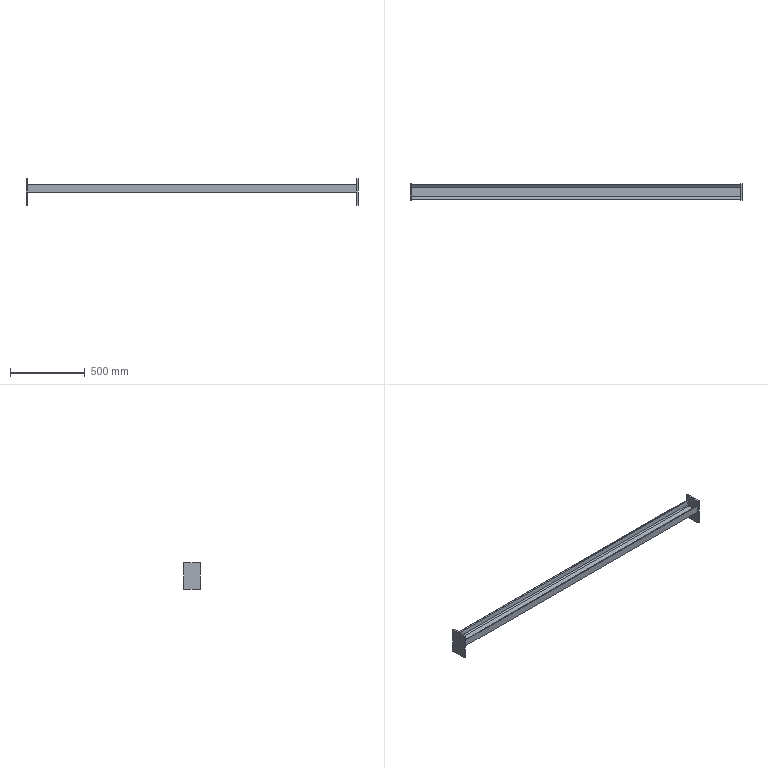Part | STEP file | Cross beam_Default<Machined> | 3 solids | 26 faces | box 2220 x 107.726 x 177.73 mm | volume 3150772 mm3 | plane 22 | cylinder 4 | commonest cylinder face diameters 8.5 x2 17 x2
STEP:
#1=CARTESIAN_POINT('',(-1100.,-100.,48.));
#2=VERTEX_POINT('',#1);
#3=CARTESIAN_POINT('',(-1100.,-100.,0.));
#4=VERTEX_POINT('',#3);
#5=CARTESIAN_POINT('',(-1100.,-100.,0.));
#6=DIRECTION('',(0.,0.,-1.));
#7=VECTOR('',#6,1000.);
#8=LINE('',#5,#7);
#9=EDGE_CURVE('',#2,#4,#8,.T.);
#10=ORIENTED_EDGE('',*,*,#9,.T.);
#11=CARTESIAN_POINT('',(1100.,-100.,0.));
#12=VERTEX_POINT('',#11);
#13=CARTESIAN_POINT('',(1100.,-100.,0.));
#14=DIRECTION('',(-1.,0.,0.));
#15=VECTOR('',#14,1000.);
#16=LINE('',#13,#15);
#17=EDGE_CURVE('',#12,#4,#16,.T.);
#18=ORIENTED_EDGE('',*,*,#17,.F.);
#19=CARTESIAN_POINT('',(1100.,-100.,48.));
#20=VERTEX_POINT('',#19);
#21=CARTESIAN_POINT('',(1100.,-100.,0.));
#22=DIRECTION('',(0.,0.,-1.));
#23=VECTOR('',#22,1000.);
#24=LINE('',#21,#23);
#25=EDGE_CURVE('',#20,#12,#24,.T.);
#26=ORIENTED_EDGE('',*,*,#25,.F.);
#27=CARTESIAN_POINT('',(1100.,-100.,48.));
#28=DIRECTION('',(-1.,0.,0.));
#29=VECTOR('',#28,1000.);
#30=LINE('',#27,#29);
#31=EDGE_CURVE('',#20,#2,#30,.T.);
#32=ORIENTED_EDGE('',*,*,#31,.T.);
#33=EDGE_LOOP('',(#10,#18,#26,#32));
#34=FACE_OUTER_BOUND('',#33,.T.);
#35=CARTESIAN_POINT('',(1100.,-100.,0.));
#36=DIRECTION('',(0.,1.,0.));
#37=DIRECTION('',(0.,0.,1.));
#38=AXIS2_PLACEMENT_3D('',#35,#36,#37);
#39=PLANE('',#38);
#40=ADVANCED_FACE('',(#34),#39,.F.);
#41=CARTESIAN_POINT('',(-1100.,0.,0.));
#42=VERTEX_POINT('',#41);
#43=CARTESIAN_POINT('',(-1100.,0.,0.));
#44=DIRECTION('',(0.,1.,0.));
#45=VECTOR('',#44,1000.);
#46=LINE('',#43,#45);
#47=EDGE_CURVE('',#4,#42,#46,.T.);
#48=ORIENTED_EDGE('',*,*,#47,.T.);
#49=CARTESIAN_POINT('',(1100.,0.,0.));
#50=VERTEX_POINT('',#49);
#51=CARTESIAN_POINT('',(1100.,0.,0.));
#52=DIRECTION('',(-1.,0.,0.));
#53=VECTOR('',#52,1000.);
#54=LINE('',#51,#53);
#55=EDGE_CURVE('',#50,#42,#54,.T.);
#56=ORIENTED_EDGE('',*,*,#55,.F.);
#57=CARTESIAN_POINT('',(1100.,0.,0.));
#58=DIRECTION('',(0.,1.,0.));
#59=VECTOR('',#58,1000.);
#60=LINE('',#57,#59);
#61=EDGE_CURVE('',#12,#50,#60,.T.);
#62=ORIENTED_EDGE('',*,*,#61,.F.);
#63=ORIENTED_EDGE('',*,*,#17,.T.);
#64=EDGE_LOOP('',(#48,#56,#62,#63));
#65=FACE_OUTER_BOUND('',#64,.T.);
#66=CARTESIAN_POINT('',(1100.,0.,0.));
#67=DIRECTION('',(0.,0.,1.));
#68=DIRECTION('',(1.,0.,0.));
#69=AXIS2_PLACEMENT_3D('',#66,#67,#68);
#70=PLANE('',#69);
#71=ADVANCED_FACE('',(#65),#70,.F.);
#72=CARTESIAN_POINT('',(-1100.,0.,48.));
#73=VERTEX_POINT('',#72);
#74=CARTESIAN_POINT('',(-1100.,0.,0.));
#75=DIRECTION('',(0.,0.,1.));
#76=VECTOR('',#75,1000.);
#77=LINE('',#74,#76);
#78=EDGE_CURVE('',#42,#73,#77,.T.);
#79=ORIENTED_EDGE('',*,*,#78,.T.);
#80=CARTESIAN_POINT('',(1100.,0.,48.));
#81=VERTEX_POINT('',#80);
#82=CARTESIAN_POINT('',(1100.,0.,48.));
#83=DIRECTION('',(-1.,0.,0.));
#84=VECTOR('',#83,1000.);
#85=LINE('',#82,#84);
#86=EDGE_CURVE('',#81,#73,#85,.T.);
#87=ORIENTED_EDGE('',*,*,#86,.F.);
#88=CARTESIAN_POINT('',(1100.,0.,0.));
#89=DIRECTION('',(0.,0.,1.));
#90=VECTOR('',#89,1000.);
#91=LINE('',#88,#90);
#92=EDGE_CURVE('',#50,#81,#91,.T.);
#93=ORIENTED_EDGE('',*,*,#92,.F.);
#94=ORIENTED_EDGE('',*,*,#55,.T.);
#95=EDGE_LOOP('',(#79,#87,#93,#94));
#96=FACE_OUTER_BOUND('',#95,.T.);
#97=CARTESIAN_POINT('',(1100.,0.,0.));
#98=DIRECTION('',(0.,-1.,0.));
#99=DIRECTION('',(0.,0.,-1.));
#100=AXIS2_PLACEMENT_3D('',#97,#98,#99);
#101=PLANE('',#100);
#102=ADVANCED_FACE('',(#96),#101,.F.);
#103=CARTESIAN_POINT('',(-1100.,-2.734,48.));
#104=VERTEX_POINT('',#103);
#105=CARTESIAN_POINT('',(-1100.,-2.734,48.));
#106=DIRECTION('',(0.,-1.,0.));
#107=VECTOR('',#106,1000.);
#108=LINE('',#105,#107);
#109=EDGE_CURVE('',#73,#104,#108,.T.);
#110=ORIENTED_EDGE('',*,*,#109,.T.);
#111=CARTESIAN_POINT('',(1100.,-2.734,48.));
#112=VERTEX_POINT('',#111);
#113=CARTESIAN_POINT('',(1100.,-2.734,48.));
#114=DIRECTION('',(-1.,0.,0.));
#115=VECTOR('',#114,1000.);
#116=LINE('',#113,#115);
#117=EDGE_CURVE('',#112,#104,#116,.T.);
#118=ORIENTED_EDGE('',*,*,#117,.F.);
#119=CARTESIAN_POINT('',(1100.,-2.734,48.));
#120=DIRECTION('',(0.,-1.,0.));
#121=VECTOR('',#120,1000.);
#122=LINE('',#119,#121);
#123=EDGE_CURVE('',#81,#112,#122,.T.);
#124=ORIENTED_EDGE('',*,*,#123,.F.);
#125=ORIENTED_EDGE('',*,*,#86,.T.);
#126=EDGE_LOOP('',(#110,#118,#124,#125));
#127=FACE_OUTER_BOUND('',#126,.T.);
#128=CARTESIAN_POINT('',(1100.,-2.734,48.));
#129=DIRECTION('',(0.,0.,-1.));
#130=DIRECTION('',(0.,1.,0.));
#131=AXIS2_PLACEMENT_3D('',#128,#129,#130);
#132=PLANE('',#131);
#133=ADVANCED_FACE('',(#127),#132,.F.);
#134=CARTESIAN_POINT('',(-1100.,-6.972,44.073));
#135=VERTEX_POINT('',#134);
#136=CARTESIAN_POINT('',(-1100.,-2.734,43.75));
#137=DIRECTION('',(1.,0.,0.));
#138=DIRECTION('',(0.,0.,-1.));
#139=AXIS2_PLACEMENT_3D('',#136,#137,#138);
#140=CIRCLE('',#139,4.25);
#141=EDGE_CURVE('',#104,#135,#140,.T.);
#142=ORIENTED_EDGE('',*,*,#141,.T.);
#143=CARTESIAN_POINT('',(1100.,-6.972,44.073));
#144=VERTEX_POINT('',#143);
#145=CARTESIAN_POINT('',(1100.,-6.972,44.073));
#146=DIRECTION('',(-1.,0.,0.));
#147=VECTOR('',#146,1000.);
#148=LINE('',#145,#147);
#149=EDGE_CURVE('',#144,#135,#148,.T.);
#150=ORIENTED_EDGE('',*,*,#149,.F.);
#151=CARTESIAN_POINT('',(1100.,-2.734,43.75));
#152=DIRECTION('',(1.,0.,0.));
#153=DIRECTION('',(0.,0.,-1.));
#154=AXIS2_PLACEMENT_3D('',#151,#152,#153);
#155=CIRCLE('',#154,4.25);
#156=EDGE_CURVE('',#112,#144,#155,.T.);
#157=ORIENTED_EDGE('',*,*,#156,.F.);
#158=ORIENTED_EDGE('',*,*,#117,.T.);
#159=EDGE_LOOP('',(#142,#150,#157,#158));
#160=FACE_OUTER_BOUND('',#159,.T.);
#161=CARTESIAN_POINT('',(1100.,-2.734,43.75));
#162=DIRECTION('',(-1.,0.,0.));
#163=DIRECTION('',(0.,0.,1.));
#164=AXIS2_PLACEMENT_3D('',#161,#162,#163);
#165=CYLINDRICAL_SURFACE('',#164,4.25);
#166=ADVANCED_FACE('',(#160),#165,.T.);
#167=CARTESIAN_POINT('',(-1100.,-9.325,13.155));
#168=VERTEX_POINT('',#167);
#169=CARTESIAN_POINT('',(-1100.,-9.325,13.155));
#170=DIRECTION('',(0.,-0.07589,-0.9971));
#171=VECTOR('',#170,1000.);
#172=LINE('',#169,#171);
#173=EDGE_CURVE('',#135,#168,#172,.T.);
#174=ORIENTED_EDGE('',*,*,#173,.T.);
#175=CARTESIAN_POINT('',(1100.,-9.325,13.155));
#176=VERTEX_POINT('',#175);
#177=CARTESIAN_POINT('',(1100.,-9.325,13.155));
#178=DIRECTION('',(-1.,0.,0.));
#179=VECTOR('',#178,1000.);
#180=LINE('',#177,#179);
#181=EDGE_CURVE('',#176,#168,#180,.T.);
#182=ORIENTED_EDGE('',*,*,#181,.F.);
#183=CARTESIAN_POINT('',(1100.,-9.325,13.155));
#184=DIRECTION('',(0.,-0.07589,-0.9971));
#185=VECTOR('',#184,1000.);
#186=LINE('',#183,#185);
#187=EDGE_CURVE('',#144,#176,#186,.T.);
#188=ORIENTED_EDGE('',*,*,#187,.F.);
#189=ORIENTED_EDGE('',*,*,#149,.T.);
#190=EDGE_LOOP('',(#174,#182,#188,#189));
#191=FACE_OUTER_BOUND('',#190,.T.);
#192=CARTESIAN_POINT('',(1100.,-9.325,13.155));
#193=DIRECTION('',(0.,0.9971,-0.07589));
#194=DIRECTION('',(0.,0.07589,0.9971));
#195=AXIS2_PLACEMENT_3D('',#192,#193,#194);
#196=PLANE('',#195);
#197=ADVANCED_FACE('',(#191),#196,.F.);
#198=CARTESIAN_POINT('',(-1100.,-17.801,5.3));
#199=VERTEX_POINT('',#198);
#200=CARTESIAN_POINT('',(-1100.,-17.801,13.8));
#201=DIRECTION('',(-1.,0.,0.));
#202=DIRECTION('',(0.,0.,1.));
#203=AXIS2_PLACEMENT_3D('',#200,#201,#202);
#204=CIRCLE('',#203,8.5);
#205=EDGE_CURVE('',#168,#199,#204,.T.);
#206=ORIENTED_EDGE('',*,*,#205,.T.);
#207=CARTESIAN_POINT('',(1100.,-17.801,5.3));
#208=VERTEX_POINT('',#207);
#209=CARTESIAN_POINT('',(1100.,-17.801,5.3));
#210=DIRECTION('',(-1.,0.,0.));
#211=VECTOR('',#210,1000.);
#212=LINE('',#209,#211);
#213=EDGE_CURVE('',#208,#199,#212,.T.);
#214=ORIENTED_EDGE('',*,*,#213,.F.);
#215=CARTESIAN_POINT('',(1100.,-17.801,13.8));
#216=DIRECTION('',(-1.,0.,0.));
#217=DIRECTION('',(0.,0.,1.));
#218=AXIS2_PLACEMENT_3D('',#215,#216,#217);
#219=CIRCLE('',#218,8.5);
#220=EDGE_CURVE('',#176,#208,#219,.T.);
#221=ORIENTED_EDGE('',*,*,#220,.F.);
#222=ORIENTED_EDGE('',*,*,#181,.T.);
#223=EDGE_LOOP('',(#206,#214,#221,#222));
#224=FACE_OUTER_BOUND('',#223,.T.);
#225=CARTESIAN_POINT('',(1100.,-17.801,13.8));
#226=DIRECTION('',(-1.,0.,0.));
#227=DIRECTION('',(0.,0.,1.));
#228=AXIS2_PLACEMENT_3D('',#225,#226,#227);
#229=CYLINDRICAL_SURFACE('',#228,8.5);
#230=ADVANCED_FACE('',(#224),#229,.F.);
#231=CARTESIAN_POINT('',(-1100.,-82.199,5.3));
#232=VERTEX_POINT('',#231);
#233=CARTESIAN_POINT('',(-1100.,-82.199,5.3));
#234=DIRECTION('',(0.,-1.,0.));
#235=VECTOR('',#234,1000.);
#236=LINE('',#233,#235);
#237=EDGE_CURVE('',#199,#232,#236,.T.);
#238=ORIENTED_EDGE('',*,*,#237,.T.);
#239=CARTESIAN_POINT('',(1100.,-82.199,5.3));
#240=VERTEX_POINT('',#239);
#241=CARTESIAN_POINT('',(1100.,-82.199,5.3));
#242=DIRECTION('',(-1.,0.,0.));
#243=VECTOR('',#242,1000.);
#244=LINE('',#241,#243);
#245=EDGE_CURVE('',#240,#232,#244,.T.);
#246=ORIENTED_EDGE('',*,*,#245,.F.);
#247=CARTESIAN_POINT('',(1100.,-82.199,5.3));
#248=DIRECTION('',(0.,-1.,0.));
#249=VECTOR('',#248,1000.);
#250=LINE('',#247,#249);
#251=EDGE_CURVE('',#208,#240,#250,.T.);
#252=ORIENTED_EDGE('',*,*,#251,.F.);
#253=ORIENTED_EDGE('',*,*,#213,.T.);
#254=EDGE_LOOP('',(#238,#246,#252,#253));
#255=FACE_OUTER_BOUND('',#254,.T.);
#256=CARTESIAN_POINT('',(1100.,-82.199,5.3));
#257=DIRECTION('',(0.,0.,-1.));
#258=DIRECTION('',(-1.,0.,0.));
#259=AXIS2_PLACEMENT_3D('',#256,#257,#258);
#260=PLANE('',#259);
#261=ADVANCED_FACE('',(#255),#260,.F.);
#262=CARTESIAN_POINT('',(-1100.,-90.675,13.155));
#263=VERTEX_POINT('',#262);
#264=CARTESIAN_POINT('',(-1100.,-82.199,13.8));
#265=DIRECTION('',(-1.,0.,0.));
#266=DIRECTION('',(0.,0.,1.));
#267=AXIS2_PLACEMENT_3D('',#264,#265,#266);
#268=CIRCLE('',#267,8.5);
#269=EDGE_CURVE('',#232,#263,#268,.T.);
#270=ORIENTED_EDGE('',*,*,#269,.T.);
#271=CARTESIAN_POINT('',(1100.,-90.675,13.155));
#272=VERTEX_POINT('',#271);
#273=CARTESIAN_POINT('',(1100.,-90.675,13.155));
#274=DIRECTION('',(-1.,0.,0.));
#275=VECTOR('',#274,1000.);
#276=LINE('',#273,#275);
#277=EDGE_CURVE('',#272,#263,#276,.T.);
#278=ORIENTED_EDGE('',*,*,#277,.F.);
#279=CARTESIAN_POINT('',(1100.,-82.199,13.8));
#280=DIRECTION('',(-1.,0.,0.));
#281=DIRECTION('',(0.,0.,1.));
#282=AXIS2_PLACEMENT_3D('',#279,#280,#281);
#283=CIRCLE('',#282,8.5);
#284=EDGE_CURVE('',#240,#272,#283,.T.);
#285=ORIENTED_EDGE('',*,*,#284,.F.);
#286=ORIENTED_EDGE('',*,*,#245,.T.);
#287=EDGE_LOOP('',(#270,#278,#285,#286));
#288=FACE_OUTER_BOUND('',#287,.T.);
#289=CARTESIAN_POINT('',(1100.,-82.199,13.8));
#290=DIRECTION('',(-1.,0.,0.));
#291=DIRECTION('',(0.,0.,1.));
#292=AXIS2_PLACEMENT_3D('',#289,#290,#291);
#293=CYLINDRICAL_SURFACE('',#292,8.5);
#294=ADVANCED_FACE('',(#288),#293,.F.);
#295=CARTESIAN_POINT('',(-1100.,-93.028,44.073));
#296=VERTEX_POINT('',#295);
#297=CARTESIAN_POINT('',(-1100.,-90.675,13.155));
#298=DIRECTION('',(0.,-0.07589,0.9971));
#299=VECTOR('',#298,1000.);
#300=LINE('',#297,#299);
#301=EDGE_CURVE('',#263,#296,#300,.T.);
#302=ORIENTED_EDGE('',*,*,#301,.T.);
#303=CARTESIAN_POINT('',(1100.,-93.028,44.073));
#304=VERTEX_POINT('',#303);
#305=CARTESIAN_POINT('',(1100.,-93.028,44.073));
#306=DIRECTION('',(-1.,0.,0.));
#307=VECTOR('',#306,1000.);
#308=LINE('',#305,#307);
#309=EDGE_CURVE('',#304,#296,#308,.T.);
#310=ORIENTED_EDGE('',*,*,#309,.F.);
#311=CARTESIAN_POINT('',(1100.,-90.675,13.155));
#312=DIRECTION('',(0.,-0.07589,0.9971));
#313=VECTOR('',#312,1000.);
#314=LINE('',#311,#313);
#315=EDGE_CURVE('',#272,#304,#314,.T.);
#316=ORIENTED_EDGE('',*,*,#315,.F.);
#317=ORIENTED_EDGE('',*,*,#277,.T.);
#318=EDGE_LOOP('',(#302,#310,#316,#317));
#319=FACE_OUTER_BOUND('',#318,.T.);
#320=CARTESIAN_POINT('',(1100.,-90.675,13.155));
#321=DIRECTION('',(0.,-0.9971,-0.07589));
#322=DIRECTION('',(0.,0.07589,-0.9971));
#323=AXIS2_PLACEMENT_3D('',#320,#321,#322);
#324=PLANE('',#323);
#325=ADVANCED_FACE('',(#319),#324,.F.);
#326=CARTESIAN_POINT('',(-1100.,-97.266,48.));
#327=VERTEX_POINT('',#326);
#328=CARTESIAN_POINT('',(-1100.,-97.266,43.75));
#329=DIRECTION('',(1.,0.,0.));
#330=DIRECTION('',(0.,0.,-1.));
#331=AXIS2_PLACEMENT_3D('',#328,#329,#330);
#332=CIRCLE('',#331,4.25);
#333=EDGE_CURVE('',#296,#327,#332,.T.);
#334=ORIENTED_EDGE('',*,*,#333,.T.);
#335=CARTESIAN_POINT('',(1100.,-97.266,48.));
#336=VERTEX_POINT('',#335);
#337=CARTESIAN_POINT('',(1100.,-97.266,48.));
#338=DIRECTION('',(-1.,0.,0.));
#339=VECTOR('',#338,1000.);
#340=LINE('',#337,#339);
#341=EDGE_CURVE('',#336,#327,#340,.T.);
#342=ORIENTED_EDGE('',*,*,#341,.F.);
#343=CARTESIAN_POINT('',(1100.,-97.266,43.75));
#344=DIRECTION('',(1.,0.,0.));
#345=DIRECTION('',(0.,0.,-1.));
#346=AXIS2_PLACEMENT_3D('',#343,#344,#345);
#347=CIRCLE('',#346,4.25);
#348=EDGE_CURVE('',#304,#336,#347,.T.);
#349=ORIENTED_EDGE('',*,*,#348,.F.);
#350=ORIENTED_EDGE('',*,*,#309,.T.);
#351=EDGE_LOOP('',(#334,#342,#349,#350));
#352=FACE_OUTER_BOUND('',#351,.T.);
#353=CARTESIAN_POINT('',(1100.,-97.266,43.75));
#354=DIRECTION('',(-1.,0.,0.));
#355=DIRECTION('',(0.,0.,1.));
#356=AXIS2_PLACEMENT_3D('',#353,#354,#355);
#357=CYLINDRICAL_SURFACE('',#356,4.25);
#358=ADVANCED_FACE('',(#352),#357,.T.);
#359=CARTESIAN_POINT('',(-1100.,-97.266,48.));
#360=DIRECTION('',(0.,-1.,0.));
#361=VECTOR('',#360,1000.);
#362=LINE('',#359,#361);
#363=EDGE_CURVE('',#327,#2,#362,.T.);
#364=ORIENTED_EDGE('',*,*,#363,.T.);
#365=ORIENTED_EDGE('',*,*,#31,.F.);
#366=CARTESIAN_POINT('',(1100.,-97.266,48.));
#367=DIRECTION('',(0.,-1.,0.));
#368=VECTOR('',#367,1000.);
#369=LINE('',#366,#368);
#370=EDGE_CURVE('',#336,#20,#369,.T.);
#371=ORIENTED_EDGE('',*,*,#370,.F.);
#372=ORIENTED_EDGE('',*,*,#341,.T.);
#373=EDGE_LOOP('',(#364,#365,#371,#372));
#374=FACE_OUTER_BOUND('',#373,.T.);
#375=CARTESIAN_POINT('',(1100.,-97.266,48.));
#376=DIRECTION('',(0.,0.,-1.));
#377=DIRECTION('',(0.,1.,0.));
#378=AXIS2_PLACEMENT_3D('',#375,#376,#377);
#379=PLANE('',#378);
#380=ADVANCED_FACE('',(#374),#379,.F.);
#381=ORIENTED_EDGE('',*,*,#25,.T.);
#382=ORIENTED_EDGE('',*,*,#61,.T.);
#383=ORIENTED_EDGE('',*,*,#92,.T.);
#384=ORIENTED_EDGE('',*,*,#123,.T.);
#385=ORIENTED_EDGE('',*,*,#156,.T.);
#386=ORIENTED_EDGE('',*,*,#187,.T.);
#387=ORIENTED_EDGE('',*,*,#220,.T.);
#388=ORIENTED_EDGE('',*,*,#251,.T.);
#389=ORIENTED_EDGE('',*,*,#284,.T.);
#390=ORIENTED_EDGE('',*,*,#315,.T.);
#391=ORIENTED_EDGE('',*,*,#348,.T.);
#392=ORIENTED_EDGE('',*,*,#370,.T.);
#393=EDGE_LOOP('',(#381,#382,#383,#384,#385,#386,#387,#388,#389,#390,#391,#392));
#394=FACE_OUTER_BOUND('',#393,.T.);
#395=CARTESIAN_POINT('',(1100.,-97.266,43.75));
#396=DIRECTION('',(1.,0.,0.));
#397=DIRECTION('',(0.,0.,-1.));
#398=AXIS2_PLACEMENT_3D('',#395,#396,#397);
#399=PLANE('',#398);
#400=ADVANCED_FACE('',(#394),#399,.T.);
#401=ORIENTED_EDGE('',*,*,#9,.F.);
#402=ORIENTED_EDGE('',*,*,#363,.F.);
#403=ORIENTED_EDGE('',*,*,#333,.F.);
#404=ORIENTED_EDGE('',*,*,#301,.F.);
#405=ORIENTED_EDGE('',*,*,#269,.F.);
#406=ORIENTED_EDGE('',*,*,#237,.F.);
#407=ORIENTED_EDGE('',*,*,#205,.F.);
#408=ORIENTED_EDGE('',*,*,#173,.F.);
#409=ORIENTED_EDGE('',*,*,#141,.F.);
#410=ORIENTED_EDGE('',*,*,#109,.F.);
#411=ORIENTED_EDGE('',*,*,#78,.F.);
#412=ORIENTED_EDGE('',*,*,#47,.F.);
#413=EDGE_LOOP('',(#401,#402,#403,#404,#405,#406,#407,#408,#409,#410,#411,#412));
#414=FACE_OUTER_BOUND('',#413,.T.);
#415=CARTESIAN_POINT('',(-1100.,-97.266,43.75));
#416=DIRECTION('',(1.,0.,0.));
#417=DIRECTION('',(0.,0.,-1.));
#418=AXIS2_PLACEMENT_3D('',#415,#416,#417);
#419=PLANE('',#418);
#420=ADVANCED_FACE('',(#414),#419,.F.);
#421=CLOSED_SHELL('',(#40,#71,#102,#133,#166,#197,#230,#261,#294,#325,#358,#380,#400,#420));
#422=MANIFOLD_SOLID_BREP('',#421);
#423=CARTESIAN_POINT('',(-1100.,-103.863,88.865));
#424=VERTEX_POINT('',#423);
#425=CARTESIAN_POINT('',(-1100.,3.863,88.865));
#426=VERTEX_POINT('',#425);
#427=CARTESIAN_POINT('',(-1100.,-103.863,88.865));
#428=DIRECTION('',(0.,1.,0.));
#429=VECTOR('',#428,1000.);
#430=LINE('',#427,#429);
#431=EDGE_CURVE('',#424,#426,#430,.T.);
#432=ORIENTED_EDGE('',*,*,#431,.T.);
#433=CARTESIAN_POINT('',(-1110.,3.863,88.865));
#434=VERTEX_POINT('',#433);
#435=CARTESIAN_POINT('',(-1110.,3.863,88.865));
#436=DIRECTION('',(1.,0.,0.));
#437=VECTOR('',#436,1000.);
#438=LINE('',#435,#437);
#439=EDGE_CURVE('',#434,#426,#438,.T.);
#440=ORIENTED_EDGE('',*,*,#439,.F.);
#441=CARTESIAN_POINT('',(-1110.,-103.863,88.865));
#442=VERTEX_POINT('',#441);
#443=CARTESIAN_POINT('',(-1110.,-103.863,88.865));
#444=DIRECTION('',(0.,1.,0.));
#445=VECTOR('',#444,1000.);
#446=LINE('',#443,#445);
#447=EDGE_CURVE('',#442,#434,#446,.T.);
#448=ORIENTED_EDGE('',*,*,#447,.F.);
#449=CARTESIAN_POINT('',(-1110.,-103.863,88.865));
#450=DIRECTION('',(1.,0.,0.));
#451=VECTOR('',#450,1000.);
#452=LINE('',#449,#451);
#453=EDGE_CURVE('',#442,#424,#452,.T.);
#454=ORIENTED_EDGE('',*,*,#453,.T.);
#455=EDGE_LOOP('',(#432,#440,#448,#454));
#456=FACE_OUTER_BOUND('',#455,.T.);
#457=CARTESIAN_POINT('',(-1110.,-103.863,88.865));
#458=DIRECTION('',(0.,0.,-1.));
#459=DIRECTION('',(-1.,0.,0.));
#460=AXIS2_PLACEMENT_3D('',#457,#458,#459);
#461=PLANE('',#460);
#462=ADVANCED_FACE('',(#456),#461,.F.);
#463=CARTESIAN_POINT('',(-1100.,3.863,-88.865));
#464=VERTEX_POINT('',#463);
#465=CARTESIAN_POINT('',(-1100.,3.863,-88.865));
#466=DIRECTION('',(0.,0.,-1.));
#467=VECTOR('',#466,1000.);
#468=LINE('',#465,#467);
#469=EDGE_CURVE('',#426,#464,#468,.T.);
#470=ORIENTED_EDGE('',*,*,#469,.T.);
#471=CARTESIAN_POINT('',(-1110.,3.863,-88.865));
#472=VERTEX_POINT('',#471);
#473=CARTESIAN_POINT('',(-1110.,3.863,-88.865));
#474=DIRECTION('',(1.,0.,0.));
#475=VECTOR('',#474,1000.);
#476=LINE('',#473,#475);
#477=EDGE_CURVE('',#472,#464,#476,.T.);
#478=ORIENTED_EDGE('',*,*,#477,.F.);
#479=CARTESIAN_POINT('',(-1110.,3.863,-88.865));
#480=DIRECTION('',(0.,0.,-1.));
#481=VECTOR('',#480,1000.);
#482=LINE('',#479,#481);
#483=EDGE_CURVE('',#434,#472,#482,.T.);
#484=ORIENTED_EDGE('',*,*,#483,.F.);
#485=ORIENTED_EDGE('',*,*,#439,.T.);
#486=EDGE_LOOP('',(#470,#478,#484,#485));
#487=FACE_OUTER_BOUND('',#486,.T.);
#488=CARTESIAN_POINT('',(-1110.,3.863,-88.865));
#489=DIRECTION('',(0.,-1.,0.));
#490=DIRECTION('',(0.,0.,-1.));
#491=AXIS2_PLACEMENT_3D('',#488,#489,#490);
#492=PLANE('',#491);
#493=ADVANCED_FACE('',(#487),#492,.F.);
#494=CARTESIAN_POINT('',(-1100.,-103.863,-88.865));
#495=VERTEX_POINT('',#494);
#496=CARTESIAN_POINT('',(-1100.,-103.863,-88.865));
#497=DIRECTION('',(0.,-1.,0.));
#498=VECTOR('',#497,1000.);
#499=LINE('',#496,#498);
#500=EDGE_CURVE('',#464,#495,#499,.T.);
#501=ORIENTED_EDGE('',*,*,#500,.T.);
#502=CARTESIAN_POINT('',(-1110.,-103.863,-88.865));
#503=VERTEX_POINT('',#502);
#504=CARTESIAN_POINT('',(-1110.,-103.863,-88.865));
#505=DIRECTION('',(1.,0.,0.));
#506=VECTOR('',#505,1000.);
#507=LINE('',#504,#506);
#508=EDGE_CURVE('',#503,#495,#507,.T.);
#509=ORIENTED_EDGE('',*,*,#508,.F.);
#510=CARTESIAN_POINT('',(-1110.,-103.863,-88.865));
#511=DIRECTION('',(0.,-1.,0.));
#512=VECTOR('',#511,1000.);
#513=LINE('',#510,#512);
#514=EDGE_CURVE('',#472,#503,#513,.T.);
#515=ORIENTED_EDGE('',*,*,#514,.F.);
#516=ORIENTED_EDGE('',*,*,#477,.T.);
#517=EDGE_LOOP('',(#501,#509,#515,#516));
#518=FACE_OUTER_BOUND('',#517,.T.);
#519=CARTESIAN_POINT('',(-1110.,-103.863,-88.865));
#520=DIRECTION('',(0.,0.,1.));
#521=DIRECTION('',(1.,0.,0.));
#522=AXIS2_PLACEMENT_3D('',#519,#520,#521);
#523=PLANE('',#522);
#524=ADVANCED_FACE('',(#518),#523,.F.);
#525=CARTESIAN_POINT('',(-1100.,-103.863,-88.865));
#526=DIRECTION('',(0.,0.,1.));
#527=VECTOR('',#526,1000.);
#528=LINE('',#525,#527);
#529=EDGE_CURVE('',#495,#424,#528,.T.);
#530=ORIENTED_EDGE('',*,*,#529,.T.);
#531=ORIENTED_EDGE('',*,*,#453,.F.);
#532=CARTESIAN_POINT('',(-1110.,-103.863,-88.865));
#533=DIRECTION('',(0.,0.,1.));
#534=VECTOR('',#533,1000.);
#535=LINE('',#532,#534);
#536=EDGE_CURVE('',#503,#442,#535,.T.);
#537=ORIENTED_EDGE('',*,*,#536,.F.);
#538=ORIENTED_EDGE('',*,*,#508,.T.);
#539=EDGE_LOOP('',(#530,#531,#537,#538));
#540=FACE_OUTER_BOUND('',#539,.T.);
#541=CARTESIAN_POINT('',(-1110.,-103.863,-88.865));
#542=DIRECTION('',(0.,1.,0.));
#543=DIRECTION('',(0.,0.,1.));
#544=AXIS2_PLACEMENT_3D('',#541,#542,#543);
#545=PLANE('',#544);
#546=ADVANCED_FACE('',(#540),#545,.F.);
#547=ORIENTED_EDGE('',*,*,#447,.T.);
#548=ORIENTED_EDGE('',*,*,#483,.T.);
#549=ORIENTED_EDGE('',*,*,#514,.T.);
#550=ORIENTED_EDGE('',*,*,#536,.T.);
#551=EDGE_LOOP('',(#547,#548,#549,#550));
#552=FACE_OUTER_BOUND('',#551,.T.);
#553=CARTESIAN_POINT('',(-1110.,0.,0.));
#554=DIRECTION('',(1.,0.,0.));
#555=DIRECTION('',(0.,0.,-1.));
#556=AXIS2_PLACEMENT_3D('',#553,#554,#555);
#557=PLANE('',#556);
#558=ADVANCED_FACE('',(#552),#557,.F.);
#559=ORIENTED_EDGE('',*,*,#431,.F.);
#560=ORIENTED_EDGE('',*,*,#529,.F.);
#561=ORIENTED_EDGE('',*,*,#500,.F.);
#562=ORIENTED_EDGE('',*,*,#469,.F.);
#563=EDGE_LOOP('',(#559,#560,#561,#562));
#564=FACE_OUTER_BOUND('',#563,.T.);
#565=CARTESIAN_POINT('',(-1100.,0.,0.));
#566=DIRECTION('',(1.,0.,0.));
#567=DIRECTION('',(0.,0.,-1.));
#568=AXIS2_PLACEMENT_3D('',#565,#566,#567);
#569=PLANE('',#568);
#570=ADVANCED_FACE('',(#564),#569,.T.);
#571=CLOSED_SHELL('',(#462,#493,#524,#546,#558,#570));
#572=MANIFOLD_SOLID_BREP('',#571);
#573=CARTESIAN_POINT('',(1100.,-103.863,88.865));
#574=VERTEX_POINT('',#573);
#575=CARTESIAN_POINT('',(1100.,3.863,88.865));
#576=VERTEX_POINT('',#575);
#577=CARTESIAN_POINT('',(1100.,-103.863,88.865));
#578=DIRECTION('',(0.,1.,0.));
#579=VECTOR('',#578,1000.);
#580=LINE('',#577,#579);
#581=EDGE_CURVE('',#574,#576,#580,.T.);
#582=ORIENTED_EDGE('',*,*,#581,.F.);
#583=CARTESIAN_POINT('',(1110.,-103.863,88.865));
#584=VERTEX_POINT('',#583);
#585=CARTESIAN_POINT('',(1110.,-103.863,88.865));
#586=DIRECTION('',(-1.,0.,0.));
#587=VECTOR('',#586,1000.);
#588=LINE('',#585,#587);
#589=EDGE_CURVE('',#584,#574,#588,.T.);
#590=ORIENTED_EDGE('',*,*,#589,.F.);
#591=CARTESIAN_POINT('',(1110.,3.863,88.865));
#592=VERTEX_POINT('',#591);
#593=CARTESIAN_POINT('',(1110.,-103.863,88.865));
#594=DIRECTION('',(0.,1.,0.));
#595=VECTOR('',#594,1000.);
#596=LINE('',#593,#595);
#597=EDGE_CURVE('',#584,#592,#596,.T.);
#598=ORIENTED_EDGE('',*,*,#597,.T.);
#599=CARTESIAN_POINT('',(1110.,3.863,88.865));
#600=DIRECTION('',(-1.,0.,0.));
#601=VECTOR('',#600,1000.);
#602=LINE('',#599,#601);
#603=EDGE_CURVE('',#592,#576,#602,.T.);
#604=ORIENTED_EDGE('',*,*,#603,.T.);
#605=EDGE_LOOP('',(#582,#590,#598,#604));
#606=FACE_OUTER_BOUND('',#605,.T.);
#607=CARTESIAN_POINT('',(1110.,-103.863,88.865));
#608=DIRECTION('',(0.,0.,-1.));
#609=DIRECTION('',(1.,0.,0.));
#610=AXIS2_PLACEMENT_3D('',#607,#608,#609);
#611=PLANE('',#610);
#612=ADVANCED_FACE('',(#606),#611,.F.);
#613=CARTESIAN_POINT('',(1100.,3.863,-88.865));
#614=VERTEX_POINT('',#613);
#615=CARTESIAN_POINT('',(1100.,3.863,-88.865));
#616=DIRECTION('',(0.,0.,-1.));
#617=VECTOR('',#616,1000.);
#618=LINE('',#615,#617);
#619=EDGE_CURVE('',#576,#614,#618,.T.);
#620=ORIENTED_EDGE('',*,*,#619,.F.);
#621=ORIENTED_EDGE('',*,*,#603,.F.);
#622=CARTESIAN_POINT('',(1110.,3.863,-88.865));
#623=VERTEX_POINT('',#622);
#624=CARTESIAN_POINT('',(1110.,3.863,-88.865));
#625=DIRECTION('',(0.,0.,-1.));
#626=VECTOR('',#625,1000.);
#627=LINE('',#624,#626);
#628=EDGE_CURVE('',#592,#623,#627,.T.);
#629=ORIENTED_EDGE('',*,*,#628,.T.);
#630=CARTESIAN_POINT('',(1110.,3.863,-88.865));
#631=DIRECTION('',(-1.,0.,0.));
#632=VECTOR('',#631,1000.);
#633=LINE('',#630,#632);
#634=EDGE_CURVE('',#623,#614,#633,.T.);
#635=ORIENTED_EDGE('',*,*,#634,.T.);
#636=EDGE_LOOP('',(#620,#621,#629,#635));
#637=FACE_OUTER_BOUND('',#636,.T.);
#638=CARTESIAN_POINT('',(1110.,3.863,-88.865));
#639=DIRECTION('',(0.,-1.,0.));
#640=DIRECTION('',(0.,0.,-1.));
#641=AXIS2_PLACEMENT_3D('',#638,#639,#640);
#642=PLANE('',#641);
#643=ADVANCED_FACE('',(#637),#642,.F.);
#644=CARTESIAN_POINT('',(1100.,-103.863,-88.865));
#645=VERTEX_POINT('',#644);
#646=CARTESIAN_POINT('',(1100.,-103.863,-88.865));
#647=DIRECTION('',(0.,-1.,0.));
#648=VECTOR('',#647,1000.);
#649=LINE('',#646,#648);
#650=EDGE_CURVE('',#614,#645,#649,.T.);
#651=ORIENTED_EDGE('',*,*,#650,.F.);
#652=ORIENTED_EDGE('',*,*,#634,.F.);
#653=CARTESIAN_POINT('',(1110.,-103.863,-88.865));
#654=VERTEX_POINT('',#653);
#655=CARTESIAN_POINT('',(1110.,-103.863,-88.865));
#656=DIRECTION('',(0.,-1.,0.));
#657=VECTOR('',#656,1000.);
#658=LINE('',#655,#657);
#659=EDGE_CURVE('',#623,#654,#658,.T.);
#660=ORIENTED_EDGE('',*,*,#659,.T.);
#661=CARTESIAN_POINT('',(1110.,-103.863,-88.865));
#662=DIRECTION('',(-1.,0.,0.));
#663=VECTOR('',#662,1000.);
#664=LINE('',#661,#663);
#665=EDGE_CURVE('',#654,#645,#664,.T.);
#666=ORIENTED_EDGE('',*,*,#665,.T.);
#667=EDGE_LOOP('',(#651,#652,#660,#666));
#668=FACE_OUTER_BOUND('',#667,.T.);
#669=CARTESIAN_POINT('',(1110.,-103.863,-88.865));
#670=DIRECTION('',(0.,0.,1.));
#671=DIRECTION('',(-1.,0.,0.));
#672=AXIS2_PLACEMENT_3D('',#669,#670,#671);
#673=PLANE('',#672);
#674=ADVANCED_FACE('',(#668),#673,.F.);
#675=CARTESIAN_POINT('',(1100.,-103.863,-88.865));
#676=DIRECTION('',(0.,0.,1.));
#677=VECTOR('',#676,1000.);
#678=LINE('',#675,#677);
#679=EDGE_CURVE('',#645,#574,#678,.T.);
#680=ORIENTED_EDGE('',*,*,#679,.F.);
#681=ORIENTED_EDGE('',*,*,#665,.F.);
#682=CARTESIAN_POINT('',(1110.,-103.863,-88.865));
#683=DIRECTION('',(0.,0.,1.));
#684=VECTOR('',#683,1000.);
#685=LINE('',#682,#684);
#686=EDGE_CURVE('',#654,#584,#685,.T.);
#687=ORIENTED_EDGE('',*,*,#686,.T.);
#688=ORIENTED_EDGE('',*,*,#589,.T.);
#689=EDGE_LOOP('',(#680,#681,#687,#688));
#690=FACE_OUTER_BOUND('',#689,.T.);
#691=CARTESIAN_POINT('',(1110.,-103.863,-88.865));
#692=DIRECTION('',(0.,1.,0.));
#693=DIRECTION('',(0.,0.,1.));
#694=AXIS2_PLACEMENT_3D('',#691,#692,#693);
#695=PLANE('',#694);
#696=ADVANCED_FACE('',(#690),#695,.F.);
#697=ORIENTED_EDGE('',*,*,#597,.F.);
#698=ORIENTED_EDGE('',*,*,#686,.F.);
#699=ORIENTED_EDGE('',*,*,#659,.F.);
#700=ORIENTED_EDGE('',*,*,#628,.F.);
#701=EDGE_LOOP('',(#697,#698,#699,#700));
#702=FACE_OUTER_BOUND('',#701,.T.);
#703=CARTESIAN_POINT('',(1110.,0.,0.));
#704=DIRECTION('',(-1.,0.,0.));
#705=DIRECTION('',(0.,0.,-1.));
#706=AXIS2_PLACEMENT_3D('',#703,#704,#705);
#707=PLANE('',#706);
#708=ADVANCED_FACE('',(#702),#707,.F.);
#709=ORIENTED_EDGE('',*,*,#581,.T.);
#710=ORIENTED_EDGE('',*,*,#619,.T.);
#711=ORIENTED_EDGE('',*,*,#650,.T.);
#712=ORIENTED_EDGE('',*,*,#679,.T.);
#713=EDGE_LOOP('',(#709,#710,#711,#712));
#714=FACE_OUTER_BOUND('',#713,.T.);
#715=CARTESIAN_POINT('',(1100.,0.,0.));
#716=DIRECTION('',(-1.,0.,0.));
#717=DIRECTION('',(0.,0.,-1.));
#718=AXIS2_PLACEMENT_3D('',#715,#716,#717);
#719=PLANE('',#718);
#720=ADVANCED_FACE('',(#714),#719,.T.);
#721=CLOSED_SHELL('',(#612,#643,#674,#696,#708,#720));
#722=MANIFOLD_SOLID_BREP('',#721);
#723=CARTESIAN_POINT('',(0.,0.,0.));
#724=DIRECTION('',(0.,0.,1.));
#725=DIRECTION('',(1.,0.,0.));
#726=AXIS2_PLACEMENT_3D('',#723,#724,#725);
#727=(LENGTH_UNIT()NAMED_UNIT(*)SI_UNIT(.MILLI.,.METRE.));
#728=UNCERTAINTY_MEASURE_WITH_UNIT(LENGTH_MEASURE(0.00001),#727,'','');
#729=(NAMED_UNIT(*)PLANE_ANGLE_UNIT()SI_UNIT($,.RADIAN.));
#730=(NAMED_UNIT(*)SI_UNIT($,.STERADIAN.)SOLID_ANGLE_UNIT());
#731=(GEOMETRIC_REPRESENTATION_CONTEXT(3)GLOBAL_UNCERTAINTY_ASSIGNED_CONTEXT((#728))GLOBAL_UNIT_ASSIGNED_CONTEXT((#727,#729,#730))REPRESENTATION_CONTEXT('',''));
#732=ADVANCED_BREP_SHAPE_REPRESENTATION('',(#422,#572,#722,#726),#731);